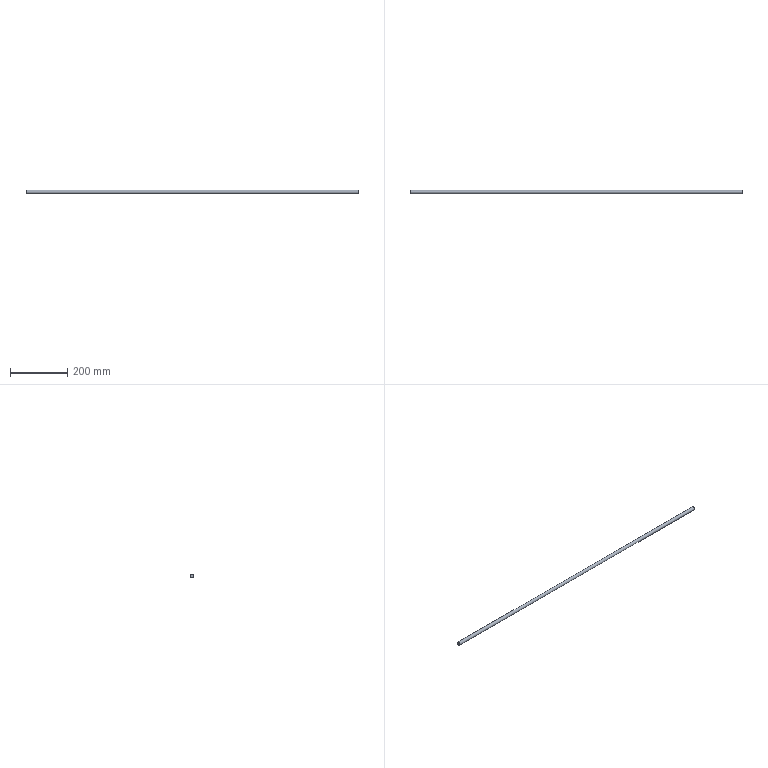Part | STEP file | solid 24 | 1 solid | 3 faces | box 1160 x 12 x 12 mm | volume 131193 mm3 | plane 2 | cylinder 1 | commonest cylinder face diameters 12 x1